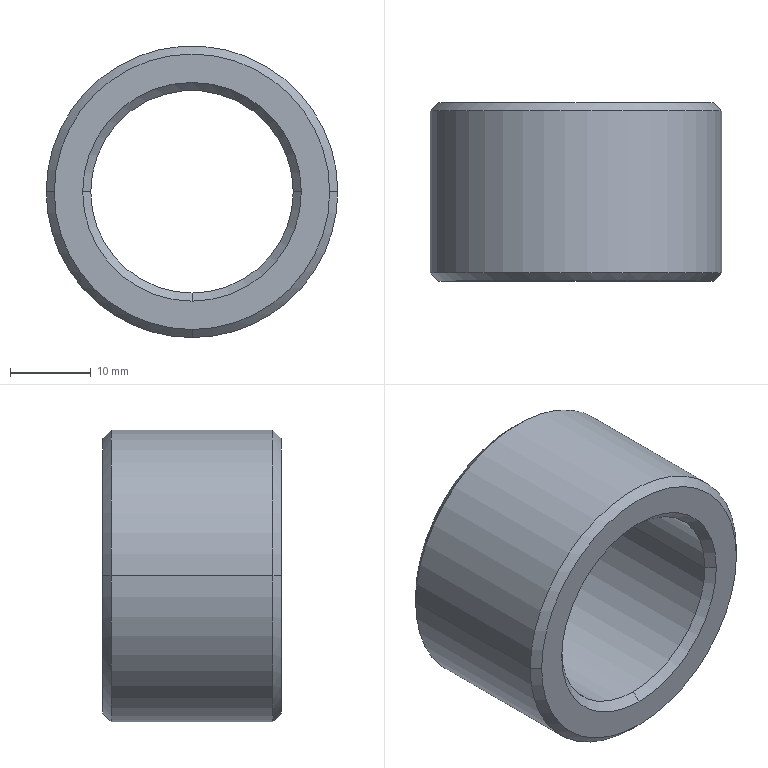Part | NX | features BREP 1 | 1 solid | 18 faces | box 36 x 22 x 36 mm | volume 11402 mm3 | cone 12 | cylinder 4 | plane 2 | commonest cylinder face diameters 25 x2 36 x2
STEP:
#1=CARTESIAN_POINT('',(-17.,0.,0.));
#2=VERTEX_POINT('',#1);
#3=CARTESIAN_POINT('',(0.,0.,-17.));
#4=VERTEX_POINT('',#3);
#5=CARTESIAN_POINT('',(0.,0.,0.));
#6=DIRECTION('',(0.,-1.,0.));
#7=DIRECTION('',(-1.,0.,0.));
#8=AXIS2_PLACEMENT_3D('',#5,#6,#7);
#9=CIRCLE('',#8,17.);
#10=EDGE_CURVE('',#2,#4,#9,.T.);
#11=ORIENTED_EDGE('',*,*,#10,.T.);
#12=CARTESIAN_POINT('',(17.,0.,0.));
#13=VERTEX_POINT('',#12);
#14=CARTESIAN_POINT('',(0.,0.,0.));
#15=DIRECTION('',(0.,-1.,0.));
#16=DIRECTION('',(-1.,0.,0.));
#17=AXIS2_PLACEMENT_3D('',#14,#15,#16);
#18=CIRCLE('',#17,17.);
#19=EDGE_CURVE('',#4,#13,#18,.T.);
#20=ORIENTED_EDGE('',*,*,#19,.T.);
#21=CARTESIAN_POINT('',(0.,0.,0.));
#22=DIRECTION('',(0.,-1.,0.));
#23=DIRECTION('',(1.,0.,0.));
#24=AXIS2_PLACEMENT_3D('',#21,#22,#23);
#25=CIRCLE('',#24,17.);
#26=EDGE_CURVE('',#13,#2,#25,.T.);
#27=ORIENTED_EDGE('',*,*,#26,.T.);
#28=EDGE_LOOP('',(#11,#20,#27));
#29=FACE_BOUND('',#28,.T.);
#30=CARTESIAN_POINT('',(13.5,0.,0.));
#31=VERTEX_POINT('',#30);
#32=CARTESIAN_POINT('',(0.,0.,-13.5));
#33=VERTEX_POINT('',#32);
#34=CARTESIAN_POINT('',(0.,0.,0.));
#35=DIRECTION('',(0.,1.,0.));
#36=DIRECTION('',(1.,0.,0.));
#37=AXIS2_PLACEMENT_3D('',#34,#35,#36);
#38=CIRCLE('',#37,13.5);
#39=EDGE_CURVE('',#31,#33,#38,.T.);
#40=ORIENTED_EDGE('',*,*,#39,.T.);
#41=CARTESIAN_POINT('',(-13.5,0.,0.));
#42=VERTEX_POINT('',#41);
#43=CARTESIAN_POINT('',(0.,0.,0.));
#44=DIRECTION('',(0.,1.,0.));
#45=DIRECTION('',(1.,0.,0.));
#46=AXIS2_PLACEMENT_3D('',#43,#44,#45);
#47=CIRCLE('',#46,13.5);
#48=EDGE_CURVE('',#33,#42,#47,.T.);
#49=ORIENTED_EDGE('',*,*,#48,.T.);
#50=CARTESIAN_POINT('',(0.,0.,0.));
#51=DIRECTION('',(0.,1.,0.));
#52=DIRECTION('',(-1.,0.,0.));
#53=AXIS2_PLACEMENT_3D('',#50,#51,#52);
#54=CIRCLE('',#53,13.5);
#55=EDGE_CURVE('',#42,#31,#54,.T.);
#56=ORIENTED_EDGE('',*,*,#55,.T.);
#57=EDGE_LOOP('',(#40,#49,#56));
#58=FACE_BOUND('',#57,.T.);
#59=CARTESIAN_POINT('',(0.,0.,0.));
#60=DIRECTION('',(0.,1.,0.));
#61=DIRECTION('',(1.,0.,0.));
#62=AXIS2_PLACEMENT_3D('',#59,#60,#61);
#63=PLANE('',#62);
#64=ADVANCED_FACE('',(#29,#58),#63,.F.);
#65=CARTESIAN_POINT('',(18.,1.,0.));
#66=VERTEX_POINT('',#65);
#67=CARTESIAN_POINT('',(17.,0.,-0.000000002));
#68=DIRECTION('',(0.7071,0.7071,0.));
#69=VECTOR('',#68,1000.);
#70=LINE('',#67,#69);
#71=EDGE_CURVE('',#13,#66,#70,.T.);
#72=ORIENTED_EDGE('',*,*,#71,.T.);
#73=CARTESIAN_POINT('',(-18.,1.,0.));
#74=VERTEX_POINT('',#73);
#75=CARTESIAN_POINT('',(0.,1.,0.));
#76=DIRECTION('',(0.,-1.,0.));
#77=DIRECTION('',(1.,0.,0.));
#78=AXIS2_PLACEMENT_3D('',#75,#76,#77);
#79=CIRCLE('',#78,18.);
#80=EDGE_CURVE('',#66,#74,#79,.T.);
#81=ORIENTED_EDGE('',*,*,#80,.T.);
#82=CARTESIAN_POINT('',(-17.,0.,0.000000002));
#83=DIRECTION('',(-0.7071,0.7071,0.));
#84=VECTOR('',#83,1000.);
#85=LINE('',#82,#84);
#86=EDGE_CURVE('',#2,#74,#85,.T.);
#87=ORIENTED_EDGE('',*,*,#86,.F.);
#88=ORIENTED_EDGE('',*,*,#26,.F.);
#89=EDGE_LOOP('',(#72,#81,#87,#88));
#90=FACE_BOUND('',#89,.T.);
#91=CARTESIAN_POINT('',(0.,0.5,0.));
#92=DIRECTION('',(0.,1.,0.));
#93=DIRECTION('',(0.,0.,-1.));
#94=AXIS2_PLACEMENT_3D('',#91,#92,#93);
#95=CONICAL_SURFACE('',#94,17.5,0.7854);
#96=ADVANCED_FACE('',(#90),#95,.T.);
#97=CARTESIAN_POINT('',(0.,1.,-18.));
#98=VERTEX_POINT('',#97);
#99=CARTESIAN_POINT('',(0.,0.5,-17.5));
#100=DIRECTION('',(0.,0.7071,-0.7071));
#101=VECTOR('',#100,1000.);
#102=LINE('',#99,#101);
#103=EDGE_CURVE('',#4,#98,#102,.T.);
#104=ORIENTED_EDGE('',*,*,#103,.F.);
#105=ORIENTED_EDGE('',*,*,#10,.F.);
#106=ORIENTED_EDGE('',*,*,#86,.T.);
#107=CARTESIAN_POINT('',(0.,1.,0.));
#108=DIRECTION('',(0.,-1.,0.));
#109=DIRECTION('',(-1.,0.,0.));
#110=AXIS2_PLACEMENT_3D('',#107,#108,#109);
#111=CIRCLE('',#110,18.);
#112=EDGE_CURVE('',#74,#98,#111,.T.);
#113=ORIENTED_EDGE('',*,*,#112,.T.);
#114=EDGE_LOOP('',(#104,#105,#106,#113));
#115=FACE_BOUND('',#114,.T.);
#116=CARTESIAN_POINT('',(0.,0.5,0.));
#117=DIRECTION('',(0.,1.,0.));
#118=DIRECTION('',(0.,0.,-1.));
#119=AXIS2_PLACEMENT_3D('',#116,#117,#118);
#120=CONICAL_SURFACE('',#119,17.5,0.7854);
#121=ADVANCED_FACE('',(#115),#120,.T.);
#122=CARTESIAN_POINT('',(18.,21.,0.));
#123=VERTEX_POINT('',#122);
#124=CARTESIAN_POINT('',(18.,1.,-0.000000002));
#125=DIRECTION('',(0.,1.,0.));
#126=VECTOR('',#125,1000.);
#127=LINE('',#124,#126);
#128=EDGE_CURVE('',#123,#66,#127,.F.);
#129=ORIENTED_EDGE('',*,*,#128,.T.);
#130=CARTESIAN_POINT('',(0.,1.,0.));
#131=DIRECTION('',(0.,-1.,0.));
#132=DIRECTION('',(-1.,0.,0.));
#133=AXIS2_PLACEMENT_3D('',#130,#131,#132);
#134=CIRCLE('',#133,18.);
#135=EDGE_CURVE('',#98,#66,#134,.T.);
#136=ORIENTED_EDGE('',*,*,#135,.F.);
#137=ORIENTED_EDGE('',*,*,#112,.F.);
#138=CARTESIAN_POINT('',(-18.,21.,0.));
#139=VERTEX_POINT('',#138);
#140=CARTESIAN_POINT('',(-18.,1.,0.000000002));
#141=DIRECTION('',(0.,1.,0.));
#142=VECTOR('',#141,1000.);
#143=LINE('',#140,#142);
#144=EDGE_CURVE('',#139,#74,#143,.F.);
#145=ORIENTED_EDGE('',*,*,#144,.F.);
#146=CARTESIAN_POINT('',(0.,21.,-18.));
#147=VERTEX_POINT('',#146);
#148=CARTESIAN_POINT('',(0.,21.,0.));
#149=DIRECTION('',(0.,1.,0.));
#150=DIRECTION('',(1.,0.,0.));
#151=AXIS2_PLACEMENT_3D('',#148,#149,#150);
#152=CIRCLE('',#151,18.);
#153=EDGE_CURVE('',#147,#139,#152,.T.);
#154=ORIENTED_EDGE('',*,*,#153,.F.);
#155=CARTESIAN_POINT('',(0.,21.,0.));
#156=DIRECTION('',(0.,1.,0.));
#157=DIRECTION('',(1.,0.,0.));
#158=AXIS2_PLACEMENT_3D('',#155,#156,#157);
#159=CIRCLE('',#158,18.);
#160=EDGE_CURVE('',#123,#147,#159,.T.);
#161=ORIENTED_EDGE('',*,*,#160,.F.);
#162=EDGE_LOOP('',(#129,#136,#137,#145,#154,#161));
#163=FACE_BOUND('',#162,.T.);
#164=CARTESIAN_POINT('',(0.,0.,0.));
#165=DIRECTION('',(0.,1.,0.));
#166=DIRECTION('',(1.,0.,0.));
#167=AXIS2_PLACEMENT_3D('',#164,#165,#166);
#168=CYLINDRICAL_SURFACE('',#167,18.);
#169=ADVANCED_FACE('',(#163),#168,.T.);
#170=CARTESIAN_POINT('',(0.,22.,-17.));
#171=VERTEX_POINT('',#170);
#172=CARTESIAN_POINT('',(0.,21.5,-17.5));
#173=DIRECTION('',(0.,-0.7071,-0.7071));
#174=VECTOR('',#173,1000.);
#175=LINE('',#172,#174);
#176=EDGE_CURVE('',#171,#147,#175,.T.);
#177=ORIENTED_EDGE('',*,*,#176,.F.);
#178=CARTESIAN_POINT('',(17.,22.,0.));
#179=VERTEX_POINT('',#178);
#180=CARTESIAN_POINT('',(0.,22.,0.));
#181=DIRECTION('',(0.,1.,0.));
#182=DIRECTION('',(1.,0.,0.));
#183=AXIS2_PLACEMENT_3D('',#180,#181,#182);
#184=CIRCLE('',#183,17.);
#185=EDGE_CURVE('',#179,#171,#184,.T.);
#186=ORIENTED_EDGE('',*,*,#185,.F.);
#187=CARTESIAN_POINT('',(17.,22.,-0.000000002));
#188=DIRECTION('',(0.7071,-0.7071,0.));
#189=VECTOR('',#188,1000.);
#190=LINE('',#187,#189);
#191=EDGE_CURVE('',#179,#123,#190,.T.);
#192=ORIENTED_EDGE('',*,*,#191,.T.);
#193=ORIENTED_EDGE('',*,*,#160,.T.);
#194=EDGE_LOOP('',(#177,#186,#192,#193));
#195=FACE_BOUND('',#194,.T.);
#196=CARTESIAN_POINT('',(0.,21.5,0.));
#197=DIRECTION('',(0.,-1.,0.));
#198=DIRECTION('',(0.,0.,-1.));
#199=AXIS2_PLACEMENT_3D('',#196,#197,#198);
#200=CONICAL_SURFACE('',#199,17.5,0.7854);
#201=ADVANCED_FACE('',(#195),#200,.T.);
#202=ORIENTED_EDGE('',*,*,#185,.T.);
#203=CARTESIAN_POINT('',(-17.,22.,0.));
#204=VERTEX_POINT('',#203);
#205=CARTESIAN_POINT('',(0.,22.,0.));
#206=DIRECTION('',(0.,1.,0.));
#207=DIRECTION('',(1.,0.,0.));
#208=AXIS2_PLACEMENT_3D('',#205,#206,#207);
#209=CIRCLE('',#208,17.);
#210=EDGE_CURVE('',#171,#204,#209,.T.);
#211=ORIENTED_EDGE('',*,*,#210,.T.);
#212=CARTESIAN_POINT('',(0.,22.,0.));
#213=DIRECTION('',(0.,1.,0.));
#214=DIRECTION('',(-1.,0.,0.));
#215=AXIS2_PLACEMENT_3D('',#212,#213,#214);
#216=CIRCLE('',#215,17.);
#217=EDGE_CURVE('',#204,#179,#216,.T.);
#218=ORIENTED_EDGE('',*,*,#217,.T.);
#219=EDGE_LOOP('',(#202,#211,#218));
#220=FACE_BOUND('',#219,.T.);
#221=CARTESIAN_POINT('',(-13.5,22.,0.));
#222=VERTEX_POINT('',#221);
#223=CARTESIAN_POINT('',(0.,22.,-13.5));
#224=VERTEX_POINT('',#223);
#225=CARTESIAN_POINT('',(0.,22.,0.));
#226=DIRECTION('',(0.,-1.,0.));
#227=DIRECTION('',(-1.,0.,0.));
#228=AXIS2_PLACEMENT_3D('',#225,#226,#227);
#229=CIRCLE('',#228,13.5);
#230=EDGE_CURVE('',#222,#224,#229,.T.);
#231=ORIENTED_EDGE('',*,*,#230,.T.);
#232=CARTESIAN_POINT('',(13.5,22.,0.));
#233=VERTEX_POINT('',#232);
#234=CARTESIAN_POINT('',(0.,22.,0.));
#235=DIRECTION('',(0.,-1.,0.));
#236=DIRECTION('',(-1.,0.,0.));
#237=AXIS2_PLACEMENT_3D('',#234,#235,#236);
#238=CIRCLE('',#237,13.5);
#239=EDGE_CURVE('',#224,#233,#238,.T.);
#240=ORIENTED_EDGE('',*,*,#239,.T.);
#241=CARTESIAN_POINT('',(0.,22.,0.));
#242=DIRECTION('',(0.,-1.,0.));
#243=DIRECTION('',(1.,0.,0.));
#244=AXIS2_PLACEMENT_3D('',#241,#242,#243);
#245=CIRCLE('',#244,13.5);
#246=EDGE_CURVE('',#233,#222,#245,.T.);
#247=ORIENTED_EDGE('',*,*,#246,.T.);
#248=EDGE_LOOP('',(#231,#240,#247));
#249=FACE_BOUND('',#248,.T.);
#250=CARTESIAN_POINT('',(0.,22.,0.));
#251=DIRECTION('',(0.,1.,0.));
#252=DIRECTION('',(1.,0.,0.));
#253=AXIS2_PLACEMENT_3D('',#250,#251,#252);
#254=PLANE('',#253);
#255=ADVANCED_FACE('',(#220,#249),#254,.T.);
#256=CARTESIAN_POINT('',(-17.,22.,0.000000002));
#257=DIRECTION('',(-0.7071,-0.7071,0.));
#258=VECTOR('',#257,1000.);
#259=LINE('',#256,#258);
#260=EDGE_CURVE('',#204,#139,#259,.T.);
#261=ORIENTED_EDGE('',*,*,#260,.T.);
#262=CARTESIAN_POINT('',(0.,21.,0.));
#263=DIRECTION('',(0.,1.,0.));
#264=DIRECTION('',(-1.,0.,0.));
#265=AXIS2_PLACEMENT_3D('',#262,#263,#264);
#266=CIRCLE('',#265,18.);
#267=EDGE_CURVE('',#139,#123,#266,.T.);
#268=ORIENTED_EDGE('',*,*,#267,.T.);
#269=ORIENTED_EDGE('',*,*,#191,.F.);
#270=ORIENTED_EDGE('',*,*,#217,.F.);
#271=EDGE_LOOP('',(#261,#268,#269,#270));
#272=FACE_BOUND('',#271,.T.);
#273=CARTESIAN_POINT('',(0.,21.5,0.));
#274=DIRECTION('',(0.,-1.,0.));
#275=DIRECTION('',(0.,0.,-1.));
#276=AXIS2_PLACEMENT_3D('',#273,#274,#275);
#277=CONICAL_SURFACE('',#276,17.5,0.7854);
#278=ADVANCED_FACE('',(#272),#277,.T.);
#279=ORIENTED_EDGE('',*,*,#144,.T.);
#280=ORIENTED_EDGE('',*,*,#80,.F.);
#281=ORIENTED_EDGE('',*,*,#128,.F.);
#282=ORIENTED_EDGE('',*,*,#267,.F.);
#283=EDGE_LOOP('',(#279,#280,#281,#282));
#284=FACE_BOUND('',#283,.T.);
#285=CARTESIAN_POINT('',(0.,0.,0.));
#286=DIRECTION('',(0.,1.,0.));
#287=DIRECTION('',(1.,0.,0.));
#288=AXIS2_PLACEMENT_3D('',#285,#286,#287);
#289=CYLINDRICAL_SURFACE('',#288,18.);
#290=ADVANCED_FACE('',(#284),#289,.T.);
#291=CARTESIAN_POINT('',(12.5,21.,0.));
#292=VERTEX_POINT('',#291);
#293=CARTESIAN_POINT('',(13.5,22.,-0.000000004));
#294=DIRECTION('',(-0.7071,-0.7071,0.000000001));
#295=VECTOR('',#294,1000.);
#296=LINE('',#293,#295);
#297=EDGE_CURVE('',#233,#292,#296,.T.);
#298=ORIENTED_EDGE('',*,*,#297,.T.);
#299=CARTESIAN_POINT('',(-12.5,21.,0.));
#300=VERTEX_POINT('',#299);
#301=CARTESIAN_POINT('',(0.,21.,0.));
#302=DIRECTION('',(0.,-1.,0.));
#303=DIRECTION('',(1.,0.,0.));
#304=AXIS2_PLACEMENT_3D('',#301,#302,#303);
#305=CIRCLE('',#304,12.5);
#306=EDGE_CURVE('',#292,#300,#305,.T.);
#307=ORIENTED_EDGE('',*,*,#306,.T.);
#308=CARTESIAN_POINT('',(-13.5,22.,0.000000004));
#309=DIRECTION('',(0.7071,-0.7071,-0.000000001));
#310=VECTOR('',#309,1000.);
#311=LINE('',#308,#310);
#312=EDGE_CURVE('',#222,#300,#311,.T.);
#313=ORIENTED_EDGE('',*,*,#312,.F.);
#314=ORIENTED_EDGE('',*,*,#246,.F.);
#315=EDGE_LOOP('',(#298,#307,#313,#314));
#316=FACE_BOUND('',#315,.T.);
#317=CARTESIAN_POINT('',(0.,21.5,0.));
#318=DIRECTION('',(0.,1.,0.));
#319=DIRECTION('',(0.,0.,-1.));
#320=AXIS2_PLACEMENT_3D('',#317,#318,#319);
#321=CONICAL_SURFACE('',#320,13.,0.7854);
#322=ADVANCED_FACE('',(#316),#321,.F.);
#323=CARTESIAN_POINT('',(0.,21.,-12.5));
#324=VERTEX_POINT('',#323);
#325=CARTESIAN_POINT('',(0.,21.5,-13.));
#326=DIRECTION('',(0.,0.7071,-0.7071));
#327=VECTOR('',#326,1000.);
#328=LINE('',#325,#327);
#329=EDGE_CURVE('',#324,#224,#328,.T.);
#330=ORIENTED_EDGE('',*,*,#329,.F.);
#331=CARTESIAN_POINT('',(0.,21.,0.));
#332=DIRECTION('',(0.,-1.,0.));
#333=DIRECTION('',(-1.,0.,0.));
#334=AXIS2_PLACEMENT_3D('',#331,#332,#333);
#335=CIRCLE('',#334,12.5);
#336=EDGE_CURVE('',#324,#292,#335,.T.);
#337=ORIENTED_EDGE('',*,*,#336,.T.);
#338=ORIENTED_EDGE('',*,*,#297,.F.);
#339=ORIENTED_EDGE('',*,*,#239,.F.);
#340=EDGE_LOOP('',(#330,#337,#338,#339));
#341=FACE_BOUND('',#340,.T.);
#342=CARTESIAN_POINT('',(0.,21.5,0.));
#343=DIRECTION('',(0.,1.,0.));
#344=DIRECTION('',(0.,0.,-1.));
#345=AXIS2_PLACEMENT_3D('',#342,#343,#344);
#346=CONICAL_SURFACE('',#345,13.,0.7854);
#347=ADVANCED_FACE('',(#341),#346,.F.);
#348=CARTESIAN_POINT('',(-12.5,1.,0.));
#349=VERTEX_POINT('',#348);
#350=CARTESIAN_POINT('',(-12.5,1.,0.000000003));
#351=DIRECTION('',(0.,1.,0.));
#352=VECTOR('',#351,1000.);
#353=LINE('',#350,#352);
#354=EDGE_CURVE('',#349,#300,#353,.T.);
#355=ORIENTED_EDGE('',*,*,#354,.F.);
#356=CARTESIAN_POINT('',(0.,1.,-12.5));
#357=VERTEX_POINT('',#356);
#358=CARTESIAN_POINT('',(0.,1.,0.));
#359=DIRECTION('',(0.,1.,0.));
#360=DIRECTION('',(1.,0.,0.));
#361=AXIS2_PLACEMENT_3D('',#358,#359,#360);
#362=CIRCLE('',#361,12.5);
#363=EDGE_CURVE('',#357,#349,#362,.T.);
#364=ORIENTED_EDGE('',*,*,#363,.F.);
#365=CARTESIAN_POINT('',(12.5,1.,0.));
#366=VERTEX_POINT('',#365);
#367=CARTESIAN_POINT('',(0.,1.,0.));
#368=DIRECTION('',(0.,1.,0.));
#369=DIRECTION('',(1.,0.,0.));
#370=AXIS2_PLACEMENT_3D('',#367,#368,#369);
#371=CIRCLE('',#370,12.5);
#372=EDGE_CURVE('',#366,#357,#371,.T.);
#373=ORIENTED_EDGE('',*,*,#372,.F.);
#374=CARTESIAN_POINT('',(12.5,1.,-0.000000003));
#375=DIRECTION('',(0.,1.,0.));
#376=VECTOR('',#375,1000.);
#377=LINE('',#374,#376);
#378=EDGE_CURVE('',#366,#292,#377,.T.);
#379=ORIENTED_EDGE('',*,*,#378,.T.);
#380=ORIENTED_EDGE('',*,*,#336,.F.);
#381=CARTESIAN_POINT('',(0.,21.,0.));
#382=DIRECTION('',(0.,-1.,0.));
#383=DIRECTION('',(-1.,0.,0.));
#384=AXIS2_PLACEMENT_3D('',#381,#382,#383);
#385=CIRCLE('',#384,12.5);
#386=EDGE_CURVE('',#300,#324,#385,.T.);
#387=ORIENTED_EDGE('',*,*,#386,.F.);
#388=EDGE_LOOP('',(#355,#364,#373,#379,#380,#387));
#389=FACE_BOUND('',#388,.T.);
#390=CARTESIAN_POINT('',(0.,0.,0.));
#391=DIRECTION('',(0.,1.,0.));
#392=DIRECTION('',(1.,0.,0.));
#393=AXIS2_PLACEMENT_3D('',#390,#391,#392);
#394=CYLINDRICAL_SURFACE('',#393,12.5);
#395=ADVANCED_FACE('',(#389),#394,.F.);
#396=ORIENTED_EDGE('',*,*,#378,.F.);
#397=CARTESIAN_POINT('',(0.,1.,0.));
#398=DIRECTION('',(0.,1.,0.));
#399=DIRECTION('',(-1.,0.,0.));
#400=AXIS2_PLACEMENT_3D('',#397,#398,#399);
#401=CIRCLE('',#400,12.5);
#402=EDGE_CURVE('',#349,#366,#401,.T.);
#403=ORIENTED_EDGE('',*,*,#402,.F.);
#404=ORIENTED_EDGE('',*,*,#354,.T.);
#405=ORIENTED_EDGE('',*,*,#306,.F.);
#406=EDGE_LOOP('',(#396,#403,#404,#405));
#407=FACE_BOUND('',#406,.T.);
#408=CARTESIAN_POINT('',(0.,0.,0.));
#409=DIRECTION('',(0.,1.,0.));
#410=DIRECTION('',(1.,0.,0.));
#411=AXIS2_PLACEMENT_3D('',#408,#409,#410);
#412=CYLINDRICAL_SURFACE('',#411,12.5);
#413=ADVANCED_FACE('',(#407),#412,.F.);
#414=CARTESIAN_POINT('',(-13.5,0.,0.000000004));
#415=DIRECTION('',(0.7071,0.7071,-0.000000001));
#416=VECTOR('',#415,1000.);
#417=LINE('',#414,#416);
#418=EDGE_CURVE('',#42,#349,#417,.T.);
#419=ORIENTED_EDGE('',*,*,#418,.T.);
#420=ORIENTED_EDGE('',*,*,#402,.T.);
#421=CARTESIAN_POINT('',(13.5,0.,-0.000000004));
#422=DIRECTION('',(-0.7071,0.7071,0.000000001));
#423=VECTOR('',#422,1000.);
#424=LINE('',#421,#423);
#425=EDGE_CURVE('',#31,#366,#424,.T.);
#426=ORIENTED_EDGE('',*,*,#425,.F.);
#427=ORIENTED_EDGE('',*,*,#55,.F.);
#428=EDGE_LOOP('',(#419,#420,#426,#427));
#429=FACE_BOUND('',#428,.T.);
#430=CARTESIAN_POINT('',(0.,0.5,0.));
#431=DIRECTION('',(0.,-1.,0.));
#432=DIRECTION('',(0.,0.,-1.));
#433=AXIS2_PLACEMENT_3D('',#430,#431,#432);
#434=CONICAL_SURFACE('',#433,13.,0.7854);
#435=ADVANCED_FACE('',(#429),#434,.F.);
#436=CARTESIAN_POINT('',(0.,0.5,-13.));
#437=DIRECTION('',(0.,-0.7071,-0.7071));
#438=VECTOR('',#437,1000.);
#439=LINE('',#436,#438);
#440=EDGE_CURVE('',#357,#33,#439,.T.);
#441=ORIENTED_EDGE('',*,*,#440,.F.);
#442=ORIENTED_EDGE('',*,*,#363,.T.);
#443=ORIENTED_EDGE('',*,*,#418,.F.);
#444=ORIENTED_EDGE('',*,*,#48,.F.);
#445=EDGE_LOOP('',(#441,#442,#443,#444));
#446=FACE_BOUND('',#445,.T.);
#447=CARTESIAN_POINT('',(0.,0.5,0.));
#448=DIRECTION('',(0.,-1.,0.));
#449=DIRECTION('',(0.,0.,-1.));
#450=AXIS2_PLACEMENT_3D('',#447,#448,#449);
#451=CONICAL_SURFACE('',#450,13.,0.7854);
#452=ADVANCED_FACE('',(#446),#451,.F.);
#453=ORIENTED_EDGE('',*,*,#372,.T.);
#454=ORIENTED_EDGE('',*,*,#440,.T.);
#455=ORIENTED_EDGE('',*,*,#39,.F.);
#456=ORIENTED_EDGE('',*,*,#425,.T.);
#457=EDGE_LOOP('',(#453,#454,#455,#456));
#458=FACE_BOUND('',#457,.T.);
#459=CARTESIAN_POINT('',(0.,0.5,0.));
#460=DIRECTION('',(0.,-1.,0.));
#461=DIRECTION('',(0.,0.,-1.));
#462=AXIS2_PLACEMENT_3D('',#459,#460,#461);
#463=CONICAL_SURFACE('',#462,13.,0.7854);
#464=ADVANCED_FACE('',(#458),#463,.F.);
#465=ORIENTED_EDGE('',*,*,#386,.T.);
#466=ORIENTED_EDGE('',*,*,#329,.T.);
#467=ORIENTED_EDGE('',*,*,#230,.F.);
#468=ORIENTED_EDGE('',*,*,#312,.T.);
#469=EDGE_LOOP('',(#465,#466,#467,#468));
#470=FACE_BOUND('',#469,.T.);
#471=CARTESIAN_POINT('',(0.,21.5,0.));
#472=DIRECTION('',(0.,1.,0.));
#473=DIRECTION('',(0.,0.,-1.));
#474=AXIS2_PLACEMENT_3D('',#471,#472,#473);
#475=CONICAL_SURFACE('',#474,13.,0.7854);
#476=ADVANCED_FACE('',(#470),#475,.F.);
#477=ORIENTED_EDGE('',*,*,#210,.F.);
#478=ORIENTED_EDGE('',*,*,#176,.T.);
#479=ORIENTED_EDGE('',*,*,#153,.T.);
#480=ORIENTED_EDGE('',*,*,#260,.F.);
#481=EDGE_LOOP('',(#477,#478,#479,#480));
#482=FACE_BOUND('',#481,.T.);
#483=CARTESIAN_POINT('',(0.,21.5,0.));
#484=DIRECTION('',(0.,-1.,0.));
#485=DIRECTION('',(0.,0.,-1.));
#486=AXIS2_PLACEMENT_3D('',#483,#484,#485);
#487=CONICAL_SURFACE('',#486,17.5,0.7854);
#488=ADVANCED_FACE('',(#482),#487,.T.);
#489=ORIENTED_EDGE('',*,*,#19,.F.);
#490=ORIENTED_EDGE('',*,*,#103,.T.);
#491=ORIENTED_EDGE('',*,*,#135,.T.);
#492=ORIENTED_EDGE('',*,*,#71,.F.);
#493=EDGE_LOOP('',(#489,#490,#491,#492));
#494=FACE_BOUND('',#493,.T.);
#495=CARTESIAN_POINT('',(0.,0.5,0.));
#496=DIRECTION('',(0.,1.,0.));
#497=DIRECTION('',(0.,0.,-1.));
#498=AXIS2_PLACEMENT_3D('',#495,#496,#497);
#499=CONICAL_SURFACE('',#498,17.5,0.7854);
#500=ADVANCED_FACE('',(#494),#499,.T.);
#501=CLOSED_SHELL('',(#64,#96,#121,#169,#201,#255,#278,#290,#322,#347,#395,#413,#435,#452,#464,#476,#488,#500));
#502=MANIFOLD_SOLID_BREP('',#501);
#503=(LENGTH_UNIT()NAMED_UNIT(*)SI_UNIT(.MILLI.,.METRE.));
#504=UNCERTAINTY_MEASURE_WITH_UNIT(LENGTH_MEASURE(0.00001),#503,'','');
#505=(NAMED_UNIT(*)PLANE_ANGLE_UNIT()SI_UNIT($,.RADIAN.));
#506=(NAMED_UNIT(*)SI_UNIT($,.STERADIAN.)SOLID_ANGLE_UNIT());
#507=(GEOMETRIC_REPRESENTATION_CONTEXT(3)GLOBAL_UNCERTAINTY_ASSIGNED_CONTEXT((#504))GLOBAL_UNIT_ASSIGNED_CONTEXT((#503,#505,#506))REPRESENTATION_CONTEXT('',''));
#508=ADVANCED_BREP_SHAPE_REPRESENTATION('',(#502),#507);